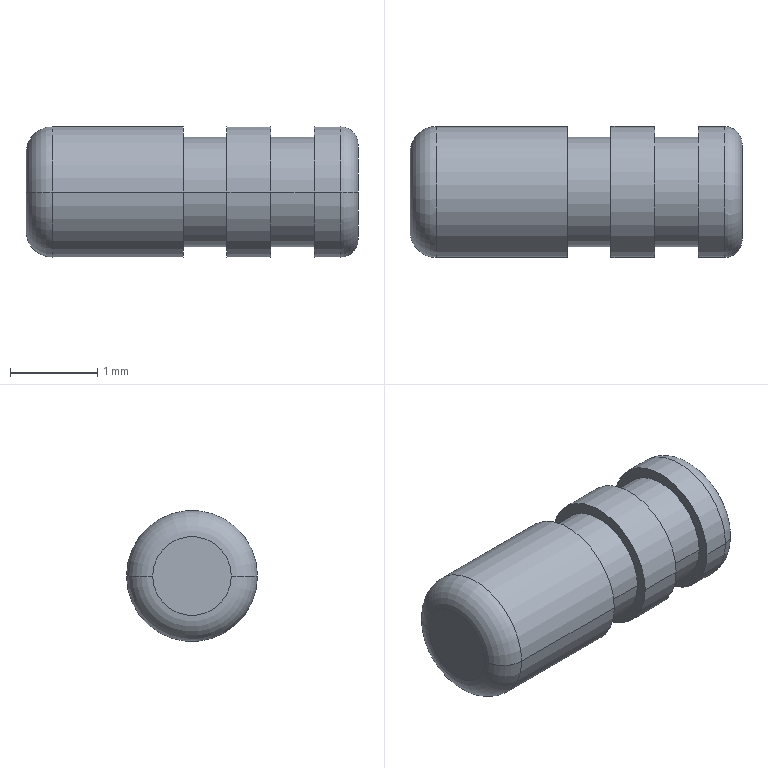Part | SolidWorks | features Revolution 1 | 1 solid | 20 faces | box 3.8 x 1.5 x 1.5 mm | volume 6.054 mm3 | cylinder 10 | plane 6 | torus 4 | commonest cylinder face diameters 1.5 x6 1.25 x4
STEP:
#1=CARTESIAN_POINT('',(-1.65,-0.75,0.));
#2=VERTEX_POINT('',#1);
#3=CARTESIAN_POINT('',(-1.65,0.75,0.));
#4=VERTEX_POINT('',#3);
#5=CARTESIAN_POINT('',(-1.65,0.,0.));
#6=DIRECTION('',(-1.,0.,0.));
#7=DIRECTION('',(0.,-1.,0.));
#8=AXIS2_PLACEMENT_3D('',#5,#6,#7);
#9=CIRCLE('',#8,0.75);
#10=EDGE_CURVE('',#2,#4,#9,.T.);
#11=ORIENTED_EDGE('',*,*,#10,.T.);
#12=CARTESIAN_POINT('',(-1.95,0.45,0.));
#13=VERTEX_POINT('',#12);
#14=CARTESIAN_POINT('',(-1.65,0.45,0.));
#15=DIRECTION('',(0.,0.,1.));
#16=DIRECTION('',(0.,-1.,0.));
#17=AXIS2_PLACEMENT_3D('',#14,#15,#16);
#18=CIRCLE('',#17,0.3);
#19=EDGE_CURVE('',#4,#13,#18,.T.);
#20=ORIENTED_EDGE('',*,*,#19,.T.);
#21=CARTESIAN_POINT('',(-1.95,-0.45,0.));
#22=VERTEX_POINT('',#21);
#23=CARTESIAN_POINT('',(-1.95,0.,0.));
#24=DIRECTION('',(-1.,0.,0.));
#25=DIRECTION('',(0.,-1.,0.));
#26=AXIS2_PLACEMENT_3D('',#23,#24,#25);
#27=CIRCLE('',#26,0.45);
#28=EDGE_CURVE('',#22,#13,#27,.T.);
#29=ORIENTED_EDGE('',*,*,#28,.F.);
#30=CARTESIAN_POINT('',(-1.65,-0.45,0.));
#31=DIRECTION('',(0.,0.,-1.));
#32=DIRECTION('',(-1.,0.,0.));
#33=AXIS2_PLACEMENT_3D('',#30,#31,#32);
#34=CIRCLE('',#33,0.3);
#35=EDGE_CURVE('',#2,#22,#34,.T.);
#36=ORIENTED_EDGE('',*,*,#35,.F.);
#37=EDGE_LOOP('',(#11,#20,#29,#36));
#38=FACE_OUTER_BOUND('',#37,.T.);
#39=CARTESIAN_POINT('',(-1.65,0.,0.));
#40=DIRECTION('',(-1.,0.,0.));
#41=DIRECTION('',(0.,-1.,0.));
#42=AXIS2_PLACEMENT_3D('',#39,#40,#41);
#43=TOROIDAL_SURFACE('',#42,0.45,0.3);
#44=ADVANCED_FACE('',(#38),#43,.T.);
#45=CARTESIAN_POINT('',(-0.15,-0.75,0.));
#46=VERTEX_POINT('',#45);
#47=CARTESIAN_POINT('',(-0.15,0.75,0.));
#48=VERTEX_POINT('',#47);
#49=CARTESIAN_POINT('',(-0.15,0.,0.));
#50=DIRECTION('',(-1.,0.,0.));
#51=DIRECTION('',(0.,-1.,0.));
#52=AXIS2_PLACEMENT_3D('',#49,#50,#51);
#53=CIRCLE('',#52,0.75);
#54=EDGE_CURVE('',#46,#48,#53,.T.);
#55=ORIENTED_EDGE('',*,*,#54,.T.);
#56=CARTESIAN_POINT('',(-2.529,0.75,0.));
#57=DIRECTION('',(-1.,0.,0.));
#58=VECTOR('',#57,1000.);
#59=LINE('',#56,#58);
#60=EDGE_CURVE('',#48,#4,#59,.T.);
#61=ORIENTED_EDGE('',*,*,#60,.T.);
#62=ORIENTED_EDGE('',*,*,#10,.F.);
#63=CARTESIAN_POINT('',(-2.529,-0.75,0.));
#64=DIRECTION('',(-1.,0.,0.));
#65=VECTOR('',#64,1000.);
#66=LINE('',#63,#65);
#67=EDGE_CURVE('',#46,#2,#66,.T.);
#68=ORIENTED_EDGE('',*,*,#67,.F.);
#69=EDGE_LOOP('',(#55,#61,#62,#68));
#70=FACE_OUTER_BOUND('',#69,.T.);
#71=CARTESIAN_POINT('',(-2.529,0.,0.));
#72=DIRECTION('',(-1.,0.,0.));
#73=DIRECTION('',(0.,-1.,0.));
#74=AXIS2_PLACEMENT_3D('',#71,#72,#73);
#75=CYLINDRICAL_SURFACE('',#74,0.75);
#76=ADVANCED_FACE('',(#70),#75,.T.);
#77=CARTESIAN_POINT('',(0.35,-0.625,0.));
#78=VERTEX_POINT('',#77);
#79=CARTESIAN_POINT('',(0.35,0.625,0.));
#80=VERTEX_POINT('',#79);
#81=CARTESIAN_POINT('',(0.35,0.,0.));
#82=DIRECTION('',(-1.,0.,0.));
#83=DIRECTION('',(0.,-1.,0.));
#84=AXIS2_PLACEMENT_3D('',#81,#82,#83);
#85=CIRCLE('',#84,0.625);
#86=EDGE_CURVE('',#78,#80,#85,.T.);
#87=ORIENTED_EDGE('',*,*,#86,.T.);
#88=CARTESIAN_POINT('',(-0.15,0.625,0.));
#89=VERTEX_POINT('',#88);
#90=CARTESIAN_POINT('',(-2.529,0.625,0.));
#91=DIRECTION('',(-1.,0.,0.));
#92=VECTOR('',#91,1000.);
#93=LINE('',#90,#92);
#94=EDGE_CURVE('',#80,#89,#93,.T.);
#95=ORIENTED_EDGE('',*,*,#94,.T.);
#96=CARTESIAN_POINT('',(-0.15,-0.625,0.));
#97=VERTEX_POINT('',#96);
#98=CARTESIAN_POINT('',(-0.15,0.,0.));
#99=DIRECTION('',(-1.,0.,0.));
#100=DIRECTION('',(0.,-1.,0.));
#101=AXIS2_PLACEMENT_3D('',#98,#99,#100);
#102=CIRCLE('',#101,0.625);
#103=EDGE_CURVE('',#97,#89,#102,.T.);
#104=ORIENTED_EDGE('',*,*,#103,.F.);
#105=CARTESIAN_POINT('',(-2.529,-0.625,0.));
#106=DIRECTION('',(-1.,0.,0.));
#107=VECTOR('',#106,1000.);
#108=LINE('',#105,#107);
#109=EDGE_CURVE('',#78,#97,#108,.T.);
#110=ORIENTED_EDGE('',*,*,#109,.F.);
#111=EDGE_LOOP('',(#87,#95,#104,#110));
#112=FACE_OUTER_BOUND('',#111,.T.);
#113=CARTESIAN_POINT('',(-2.529,0.,0.));
#114=DIRECTION('',(-1.,0.,0.));
#115=DIRECTION('',(0.,-1.,0.));
#116=AXIS2_PLACEMENT_3D('',#113,#114,#115);
#117=CYLINDRICAL_SURFACE('',#116,0.625);
#118=ADVANCED_FACE('',(#112),#117,.T.);
#119=CARTESIAN_POINT('',(0.85,-0.75,0.));
#120=VERTEX_POINT('',#119);
#121=CARTESIAN_POINT('',(0.85,0.75,0.));
#122=VERTEX_POINT('',#121);
#123=CARTESIAN_POINT('',(0.85,0.,0.));
#124=DIRECTION('',(-1.,0.,0.));
#125=DIRECTION('',(0.,-1.,0.));
#126=AXIS2_PLACEMENT_3D('',#123,#124,#125);
#127=CIRCLE('',#126,0.75);
#128=EDGE_CURVE('',#120,#122,#127,.T.);
#129=ORIENTED_EDGE('',*,*,#128,.T.);
#130=CARTESIAN_POINT('',(0.35,0.75,0.));
#131=VERTEX_POINT('',#130);
#132=CARTESIAN_POINT('',(-2.529,0.75,0.));
#133=DIRECTION('',(-1.,0.,0.));
#134=VECTOR('',#133,1000.);
#135=LINE('',#132,#134);
#136=EDGE_CURVE('',#122,#131,#135,.T.);
#137=ORIENTED_EDGE('',*,*,#136,.T.);
#138=CARTESIAN_POINT('',(0.35,-0.75,0.));
#139=VERTEX_POINT('',#138);
#140=CARTESIAN_POINT('',(0.35,0.,0.));
#141=DIRECTION('',(-1.,0.,0.));
#142=DIRECTION('',(0.,-1.,0.));
#143=AXIS2_PLACEMENT_3D('',#140,#141,#142);
#144=CIRCLE('',#143,0.75);
#145=EDGE_CURVE('',#139,#131,#144,.T.);
#146=ORIENTED_EDGE('',*,*,#145,.F.);
#147=CARTESIAN_POINT('',(-2.529,-0.75,0.));
#148=DIRECTION('',(-1.,0.,0.));
#149=VECTOR('',#148,1000.);
#150=LINE('',#147,#149);
#151=EDGE_CURVE('',#120,#139,#150,.T.);
#152=ORIENTED_EDGE('',*,*,#151,.F.);
#153=EDGE_LOOP('',(#129,#137,#146,#152));
#154=FACE_OUTER_BOUND('',#153,.T.);
#155=CARTESIAN_POINT('',(-2.529,0.,0.));
#156=DIRECTION('',(-1.,0.,0.));
#157=DIRECTION('',(0.,-1.,0.));
#158=AXIS2_PLACEMENT_3D('',#155,#156,#157);
#159=CYLINDRICAL_SURFACE('',#158,0.75);
#160=ADVANCED_FACE('',(#154),#159,.T.);
#161=CARTESIAN_POINT('',(1.35,-0.625,0.));
#162=VERTEX_POINT('',#161);
#163=CARTESIAN_POINT('',(1.35,0.625,0.));
#164=VERTEX_POINT('',#163);
#165=CARTESIAN_POINT('',(1.35,0.,0.));
#166=DIRECTION('',(-1.,0.,0.));
#167=DIRECTION('',(0.,-1.,0.));
#168=AXIS2_PLACEMENT_3D('',#165,#166,#167);
#169=CIRCLE('',#168,0.625);
#170=EDGE_CURVE('',#162,#164,#169,.T.);
#171=ORIENTED_EDGE('',*,*,#170,.T.);
#172=CARTESIAN_POINT('',(0.85,0.625,0.));
#173=VERTEX_POINT('',#172);
#174=CARTESIAN_POINT('',(-2.529,0.625,0.));
#175=DIRECTION('',(-1.,0.,0.));
#176=VECTOR('',#175,1000.);
#177=LINE('',#174,#176);
#178=EDGE_CURVE('',#164,#173,#177,.T.);
#179=ORIENTED_EDGE('',*,*,#178,.T.);
#180=CARTESIAN_POINT('',(0.85,-0.625,0.));
#181=VERTEX_POINT('',#180);
#182=CARTESIAN_POINT('',(0.85,0.,0.));
#183=DIRECTION('',(-1.,0.,0.));
#184=DIRECTION('',(0.,-1.,0.));
#185=AXIS2_PLACEMENT_3D('',#182,#183,#184);
#186=CIRCLE('',#185,0.625);
#187=EDGE_CURVE('',#181,#173,#186,.T.);
#188=ORIENTED_EDGE('',*,*,#187,.F.);
#189=CARTESIAN_POINT('',(-2.529,-0.625,0.));
#190=DIRECTION('',(-1.,0.,0.));
#191=VECTOR('',#190,1000.);
#192=LINE('',#189,#191);
#193=EDGE_CURVE('',#162,#181,#192,.T.);
#194=ORIENTED_EDGE('',*,*,#193,.F.);
#195=EDGE_LOOP('',(#171,#179,#188,#194));
#196=FACE_OUTER_BOUND('',#195,.T.);
#197=CARTESIAN_POINT('',(-2.529,0.,0.));
#198=DIRECTION('',(-1.,0.,0.));
#199=DIRECTION('',(0.,-1.,0.));
#200=AXIS2_PLACEMENT_3D('',#197,#198,#199);
#201=CYLINDRICAL_SURFACE('',#200,0.625);
#202=ADVANCED_FACE('',(#196),#201,.T.);
#203=CARTESIAN_POINT('',(1.65,-0.75,0.));
#204=VERTEX_POINT('',#203);
#205=CARTESIAN_POINT('',(1.65,0.75,0.));
#206=VERTEX_POINT('',#205);
#207=CARTESIAN_POINT('',(1.65,0.,0.));
#208=DIRECTION('',(-1.,0.,0.));
#209=DIRECTION('',(0.,-1.,0.));
#210=AXIS2_PLACEMENT_3D('',#207,#208,#209);
#211=CIRCLE('',#210,0.75);
#212=EDGE_CURVE('',#204,#206,#211,.T.);
#213=ORIENTED_EDGE('',*,*,#212,.T.);
#214=CARTESIAN_POINT('',(1.35,0.75,0.));
#215=VERTEX_POINT('',#214);
#216=CARTESIAN_POINT('',(-2.529,0.75,0.));
#217=DIRECTION('',(-1.,0.,0.));
#218=VECTOR('',#217,1000.);
#219=LINE('',#216,#218);
#220=EDGE_CURVE('',#206,#215,#219,.T.);
#221=ORIENTED_EDGE('',*,*,#220,.T.);
#222=CARTESIAN_POINT('',(1.35,-0.75,0.));
#223=VERTEX_POINT('',#222);
#224=CARTESIAN_POINT('',(1.35,0.,0.));
#225=DIRECTION('',(-1.,0.,0.));
#226=DIRECTION('',(0.,-1.,0.));
#227=AXIS2_PLACEMENT_3D('',#224,#225,#226);
#228=CIRCLE('',#227,0.75);
#229=EDGE_CURVE('',#223,#215,#228,.T.);
#230=ORIENTED_EDGE('',*,*,#229,.F.);
#231=CARTESIAN_POINT('',(-2.529,-0.75,0.));
#232=DIRECTION('',(-1.,0.,0.));
#233=VECTOR('',#232,1000.);
#234=LINE('',#231,#233);
#235=EDGE_CURVE('',#204,#223,#234,.T.);
#236=ORIENTED_EDGE('',*,*,#235,.F.);
#237=EDGE_LOOP('',(#213,#221,#230,#236));
#238=FACE_OUTER_BOUND('',#237,.T.);
#239=CARTESIAN_POINT('',(-2.529,0.,0.));
#240=DIRECTION('',(-1.,0.,0.));
#241=DIRECTION('',(0.,-1.,0.));
#242=AXIS2_PLACEMENT_3D('',#239,#240,#241);
#243=CYLINDRICAL_SURFACE('',#242,0.75);
#244=ADVANCED_FACE('',(#238),#243,.T.);
#245=CARTESIAN_POINT('',(1.85,-0.55,0.));
#246=VERTEX_POINT('',#245);
#247=CARTESIAN_POINT('',(1.85,0.55,0.));
#248=VERTEX_POINT('',#247);
#249=CARTESIAN_POINT('',(1.85,0.,0.));
#250=DIRECTION('',(-1.,0.,0.));
#251=DIRECTION('',(0.,-1.,0.));
#252=AXIS2_PLACEMENT_3D('',#249,#250,#251);
#253=CIRCLE('',#252,0.55);
#254=EDGE_CURVE('',#246,#248,#253,.T.);
#255=ORIENTED_EDGE('',*,*,#254,.T.);
#256=CARTESIAN_POINT('',(1.65,0.55,0.));
#257=DIRECTION('',(0.,0.,1.));
#258=DIRECTION('',(0.,-1.,0.));
#259=AXIS2_PLACEMENT_3D('',#256,#257,#258);
#260=CIRCLE('',#259,0.2);
#261=EDGE_CURVE('',#248,#206,#260,.T.);
#262=ORIENTED_EDGE('',*,*,#261,.T.);
#263=ORIENTED_EDGE('',*,*,#212,.F.);
#264=CARTESIAN_POINT('',(1.65,-0.55,0.));
#265=DIRECTION('',(0.,0.,-1.));
#266=DIRECTION('',(-1.,0.,0.));
#267=AXIS2_PLACEMENT_3D('',#264,#265,#266);
#268=CIRCLE('',#267,0.2);
#269=EDGE_CURVE('',#246,#204,#268,.T.);
#270=ORIENTED_EDGE('',*,*,#269,.F.);
#271=EDGE_LOOP('',(#255,#262,#263,#270));
#272=FACE_OUTER_BOUND('',#271,.T.);
#273=CARTESIAN_POINT('',(1.65,0.,0.));
#274=DIRECTION('',(-1.,0.,0.));
#275=DIRECTION('',(0.,-1.,0.));
#276=AXIS2_PLACEMENT_3D('',#273,#274,#275);
#277=TOROIDAL_SURFACE('',#276,0.55,0.2);
#278=ADVANCED_FACE('',(#272),#277,.T.);
#279=ORIENTED_EDGE('',*,*,#254,.F.);
#280=CARTESIAN_POINT('',(1.85,0.,0.));
#281=DIRECTION('',(-1.,0.,0.));
#282=DIRECTION('',(0.,-1.,0.));
#283=AXIS2_PLACEMENT_3D('',#280,#281,#282);
#284=CIRCLE('',#283,0.55);
#285=EDGE_CURVE('',#248,#246,#284,.T.);
#286=ORIENTED_EDGE('',*,*,#285,.F.);
#287=EDGE_LOOP('',(#279,#286));
#288=FACE_OUTER_BOUND('',#287,.T.);
#289=CARTESIAN_POINT('',(1.85,0.55,0.));
#290=DIRECTION('',(-1.,0.,0.));
#291=DIRECTION('',(0.,-1.,0.));
#292=AXIS2_PLACEMENT_3D('',#289,#290,#291);
#293=PLANE('',#292);
#294=ADVANCED_FACE('',(#288),#293,.F.);
#295=ORIENTED_EDGE('',*,*,#261,.F.);
#296=ORIENTED_EDGE('',*,*,#285,.T.);
#297=ORIENTED_EDGE('',*,*,#269,.T.);
#298=CARTESIAN_POINT('',(1.65,0.,0.));
#299=DIRECTION('',(-1.,0.,0.));
#300=DIRECTION('',(0.,-1.,0.));
#301=AXIS2_PLACEMENT_3D('',#298,#299,#300);
#302=CIRCLE('',#301,0.75);
#303=EDGE_CURVE('',#206,#204,#302,.T.);
#304=ORIENTED_EDGE('',*,*,#303,.F.);
#305=EDGE_LOOP('',(#295,#296,#297,#304));
#306=FACE_OUTER_BOUND('',#305,.T.);
#307=CARTESIAN_POINT('',(1.65,0.,0.));
#308=DIRECTION('',(-1.,0.,0.));
#309=DIRECTION('',(0.,-1.,0.));
#310=AXIS2_PLACEMENT_3D('',#307,#308,#309);
#311=TOROIDAL_SURFACE('',#310,0.55,0.2);
#312=ADVANCED_FACE('',(#306),#311,.T.);
#313=ORIENTED_EDGE('',*,*,#220,.F.);
#314=ORIENTED_EDGE('',*,*,#303,.T.);
#315=ORIENTED_EDGE('',*,*,#235,.T.);
#316=CARTESIAN_POINT('',(1.35,0.,0.));
#317=DIRECTION('',(-1.,0.,0.));
#318=DIRECTION('',(0.,-1.,0.));
#319=AXIS2_PLACEMENT_3D('',#316,#317,#318);
#320=CIRCLE('',#319,0.75);
#321=EDGE_CURVE('',#215,#223,#320,.T.);
#322=ORIENTED_EDGE('',*,*,#321,.F.);
#323=EDGE_LOOP('',(#313,#314,#315,#322));
#324=FACE_OUTER_BOUND('',#323,.T.);
#325=CARTESIAN_POINT('',(-2.529,0.,0.));
#326=DIRECTION('',(-1.,0.,0.));
#327=DIRECTION('',(0.,-1.,0.));
#328=AXIS2_PLACEMENT_3D('',#325,#326,#327);
#329=CYLINDRICAL_SURFACE('',#328,0.75);
#330=ADVANCED_FACE('',(#324),#329,.T.);
#331=ORIENTED_EDGE('',*,*,#170,.F.);
#332=CARTESIAN_POINT('',(1.35,0.,0.));
#333=DIRECTION('',(-1.,0.,0.));
#334=DIRECTION('',(0.,-1.,0.));
#335=AXIS2_PLACEMENT_3D('',#332,#333,#334);
#336=CIRCLE('',#335,0.625);
#337=EDGE_CURVE('',#164,#162,#336,.T.);
#338=ORIENTED_EDGE('',*,*,#337,.F.);
#339=EDGE_LOOP('',(#331,#338));
#340=FACE_BOUND('',#339,.T.);
#341=ORIENTED_EDGE('',*,*,#229,.T.);
#342=ORIENTED_EDGE('',*,*,#321,.T.);
#343=EDGE_LOOP('',(#341,#342));
#344=FACE_OUTER_BOUND('',#343,.T.);
#345=CARTESIAN_POINT('',(1.35,0.75,0.));
#346=DIRECTION('',(1.,0.,0.));
#347=DIRECTION('',(0.,1.,0.));
#348=AXIS2_PLACEMENT_3D('',#345,#346,#347);
#349=PLANE('',#348);
#350=ADVANCED_FACE('',(#340,#344),#349,.F.);
#351=ORIENTED_EDGE('',*,*,#178,.F.);
#352=ORIENTED_EDGE('',*,*,#337,.T.);
#353=ORIENTED_EDGE('',*,*,#193,.T.);
#354=CARTESIAN_POINT('',(0.85,0.,0.));
#355=DIRECTION('',(-1.,0.,0.));
#356=DIRECTION('',(0.,-1.,0.));
#357=AXIS2_PLACEMENT_3D('',#354,#355,#356);
#358=CIRCLE('',#357,0.625);
#359=EDGE_CURVE('',#173,#181,#358,.T.);
#360=ORIENTED_EDGE('',*,*,#359,.F.);
#361=EDGE_LOOP('',(#351,#352,#353,#360));
#362=FACE_OUTER_BOUND('',#361,.T.);
#363=CARTESIAN_POINT('',(-2.529,0.,0.));
#364=DIRECTION('',(-1.,0.,0.));
#365=DIRECTION('',(0.,-1.,0.));
#366=AXIS2_PLACEMENT_3D('',#363,#364,#365);
#367=CYLINDRICAL_SURFACE('',#366,0.625);
#368=ADVANCED_FACE('',(#362),#367,.T.);
#369=ORIENTED_EDGE('',*,*,#128,.F.);
#370=CARTESIAN_POINT('',(0.85,0.,0.));
#371=DIRECTION('',(-1.,0.,0.));
#372=DIRECTION('',(0.,-1.,0.));
#373=AXIS2_PLACEMENT_3D('',#370,#371,#372);
#374=CIRCLE('',#373,0.75);
#375=EDGE_CURVE('',#122,#120,#374,.T.);
#376=ORIENTED_EDGE('',*,*,#375,.F.);
#377=EDGE_LOOP('',(#369,#376));
#378=FACE_OUTER_BOUND('',#377,.T.);
#379=ORIENTED_EDGE('',*,*,#187,.T.);
#380=ORIENTED_EDGE('',*,*,#359,.T.);
#381=EDGE_LOOP('',(#379,#380));
#382=FACE_BOUND('',#381,.T.);
#383=CARTESIAN_POINT('',(0.85,0.625,0.));
#384=DIRECTION('',(-1.,0.,0.));
#385=DIRECTION('',(0.,-1.,0.));
#386=AXIS2_PLACEMENT_3D('',#383,#384,#385);
#387=PLANE('',#386);
#388=ADVANCED_FACE('',(#378,#382),#387,.F.);
#389=ORIENTED_EDGE('',*,*,#136,.F.);
#390=ORIENTED_EDGE('',*,*,#375,.T.);
#391=ORIENTED_EDGE('',*,*,#151,.T.);
#392=CARTESIAN_POINT('',(0.35,0.,0.));
#393=DIRECTION('',(-1.,0.,0.));
#394=DIRECTION('',(0.,-1.,0.));
#395=AXIS2_PLACEMENT_3D('',#392,#393,#394);
#396=CIRCLE('',#395,0.75);
#397=EDGE_CURVE('',#131,#139,#396,.T.);
#398=ORIENTED_EDGE('',*,*,#397,.F.);
#399=EDGE_LOOP('',(#389,#390,#391,#398));
#400=FACE_OUTER_BOUND('',#399,.T.);
#401=CARTESIAN_POINT('',(-2.529,0.,0.));
#402=DIRECTION('',(-1.,0.,0.));
#403=DIRECTION('',(0.,-1.,0.));
#404=AXIS2_PLACEMENT_3D('',#401,#402,#403);
#405=CYLINDRICAL_SURFACE('',#404,0.75);
#406=ADVANCED_FACE('',(#400),#405,.T.);
#407=ORIENTED_EDGE('',*,*,#86,.F.);
#408=CARTESIAN_POINT('',(0.35,0.,0.));
#409=DIRECTION('',(-1.,0.,0.));
#410=DIRECTION('',(0.,-1.,0.));
#411=AXIS2_PLACEMENT_3D('',#408,#409,#410);
#412=CIRCLE('',#411,0.625);
#413=EDGE_CURVE('',#80,#78,#412,.T.);
#414=ORIENTED_EDGE('',*,*,#413,.F.);
#415=EDGE_LOOP('',(#407,#414));
#416=FACE_BOUND('',#415,.T.);
#417=ORIENTED_EDGE('',*,*,#145,.T.);
#418=ORIENTED_EDGE('',*,*,#397,.T.);
#419=EDGE_LOOP('',(#417,#418));
#420=FACE_OUTER_BOUND('',#419,.T.);
#421=CARTESIAN_POINT('',(0.35,0.625,0.));
#422=DIRECTION('',(1.,0.,0.));
#423=DIRECTION('',(0.,1.,0.));
#424=AXIS2_PLACEMENT_3D('',#421,#422,#423);
#425=PLANE('',#424);
#426=ADVANCED_FACE('',(#416,#420),#425,.F.);
#427=ORIENTED_EDGE('',*,*,#94,.F.);
#428=ORIENTED_EDGE('',*,*,#413,.T.);
#429=ORIENTED_EDGE('',*,*,#109,.T.);
#430=CARTESIAN_POINT('',(-0.15,0.,0.));
#431=DIRECTION('',(-1.,0.,0.));
#432=DIRECTION('',(0.,-1.,0.));
#433=AXIS2_PLACEMENT_3D('',#430,#431,#432);
#434=CIRCLE('',#433,0.625);
#435=EDGE_CURVE('',#89,#97,#434,.T.);
#436=ORIENTED_EDGE('',*,*,#435,.F.);
#437=EDGE_LOOP('',(#427,#428,#429,#436));
#438=FACE_OUTER_BOUND('',#437,.T.);
#439=CARTESIAN_POINT('',(-2.529,0.,0.));
#440=DIRECTION('',(-1.,0.,0.));
#441=DIRECTION('',(0.,-1.,0.));
#442=AXIS2_PLACEMENT_3D('',#439,#440,#441);
#443=CYLINDRICAL_SURFACE('',#442,0.625);
#444=ADVANCED_FACE('',(#438),#443,.T.);
#445=ORIENTED_EDGE('',*,*,#54,.F.);
#446=CARTESIAN_POINT('',(-0.15,0.,0.));
#447=DIRECTION('',(-1.,0.,0.));
#448=DIRECTION('',(0.,-1.,0.));
#449=AXIS2_PLACEMENT_3D('',#446,#447,#448);
#450=CIRCLE('',#449,0.75);
#451=EDGE_CURVE('',#48,#46,#450,.T.);
#452=ORIENTED_EDGE('',*,*,#451,.F.);
#453=EDGE_LOOP('',(#445,#452));
#454=FACE_OUTER_BOUND('',#453,.T.);
#455=ORIENTED_EDGE('',*,*,#103,.T.);
#456=ORIENTED_EDGE('',*,*,#435,.T.);
#457=EDGE_LOOP('',(#455,#456));
#458=FACE_BOUND('',#457,.T.);
#459=CARTESIAN_POINT('',(-0.15,0.75,0.));
#460=DIRECTION('',(-1.,0.,0.));
#461=DIRECTION('',(0.,-1.,0.));
#462=AXIS2_PLACEMENT_3D('',#459,#460,#461);
#463=PLANE('',#462);
#464=ADVANCED_FACE('',(#454,#458),#463,.F.);
#465=ORIENTED_EDGE('',*,*,#60,.F.);
#466=ORIENTED_EDGE('',*,*,#451,.T.);
#467=ORIENTED_EDGE('',*,*,#67,.T.);
#468=CARTESIAN_POINT('',(-1.65,0.,0.));
#469=DIRECTION('',(-1.,0.,0.));
#470=DIRECTION('',(0.,-1.,0.));
#471=AXIS2_PLACEMENT_3D('',#468,#469,#470);
#472=CIRCLE('',#471,0.75);
#473=EDGE_CURVE('',#4,#2,#472,.T.);
#474=ORIENTED_EDGE('',*,*,#473,.F.);
#475=EDGE_LOOP('',(#465,#466,#467,#474));
#476=FACE_OUTER_BOUND('',#475,.T.);
#477=CARTESIAN_POINT('',(-2.529,0.,0.));
#478=DIRECTION('',(-1.,0.,0.));
#479=DIRECTION('',(0.,-1.,0.));
#480=AXIS2_PLACEMENT_3D('',#477,#478,#479);
#481=CYLINDRICAL_SURFACE('',#480,0.75);
#482=ADVANCED_FACE('',(#476),#481,.T.);
#483=ORIENTED_EDGE('',*,*,#19,.F.);
#484=ORIENTED_EDGE('',*,*,#473,.T.);
#485=ORIENTED_EDGE('',*,*,#35,.T.);
#486=CARTESIAN_POINT('',(-1.95,0.,0.));
#487=DIRECTION('',(-1.,0.,0.));
#488=DIRECTION('',(0.,-1.,0.));
#489=AXIS2_PLACEMENT_3D('',#486,#487,#488);
#490=CIRCLE('',#489,0.45);
#491=EDGE_CURVE('',#13,#22,#490,.T.);
#492=ORIENTED_EDGE('',*,*,#491,.F.);
#493=EDGE_LOOP('',(#483,#484,#485,#492));
#494=FACE_OUTER_BOUND('',#493,.T.);
#495=CARTESIAN_POINT('',(-1.65,0.,0.));
#496=DIRECTION('',(-1.,0.,0.));
#497=DIRECTION('',(0.,-1.,0.));
#498=AXIS2_PLACEMENT_3D('',#495,#496,#497);
#499=TOROIDAL_SURFACE('',#498,0.45,0.3);
#500=ADVANCED_FACE('',(#494),#499,.T.);
#501=ORIENTED_EDGE('',*,*,#28,.T.);
#502=ORIENTED_EDGE('',*,*,#491,.T.);
#503=EDGE_LOOP('',(#501,#502));
#504=FACE_OUTER_BOUND('',#503,.T.);
#505=CARTESIAN_POINT('',(-1.95,0.45,0.));
#506=DIRECTION('',(1.,0.,0.));
#507=DIRECTION('',(0.,1.,0.));
#508=AXIS2_PLACEMENT_3D('',#505,#506,#507);
#509=PLANE('',#508);
#510=ADVANCED_FACE('',(#504),#509,.F.);
#511=CLOSED_SHELL('',(#44,#76,#118,#160,#202,#244,#278,#294,#312,#330,#350,#368,#388,#406,#426,#444,#464,#482,#500,#510));
#512=MANIFOLD_SOLID_BREP('',#511);
#513=CARTESIAN_POINT('',(0.,0.,0.));
#514=DIRECTION('',(0.,0.,1.));
#515=DIRECTION('',(1.,0.,0.));
#516=AXIS2_PLACEMENT_3D('',#513,#514,#515);
#517=(LENGTH_UNIT()NAMED_UNIT(*)SI_UNIT(.MILLI.,.METRE.));
#518=UNCERTAINTY_MEASURE_WITH_UNIT(LENGTH_MEASURE(0.00001),#517,'','');
#519=(NAMED_UNIT(*)PLANE_ANGLE_UNIT()SI_UNIT($,.RADIAN.));
#520=(NAMED_UNIT(*)SI_UNIT($,.STERADIAN.)SOLID_ANGLE_UNIT());
#521=(GEOMETRIC_REPRESENTATION_CONTEXT(3)GLOBAL_UNCERTAINTY_ASSIGNED_CONTEXT((#518))GLOBAL_UNIT_ASSIGNED_CONTEXT((#517,#519,#520))REPRESENTATION_CONTEXT('',''));
#522=ADVANCED_BREP_SHAPE_REPRESENTATION('',(#512,#516),#521);